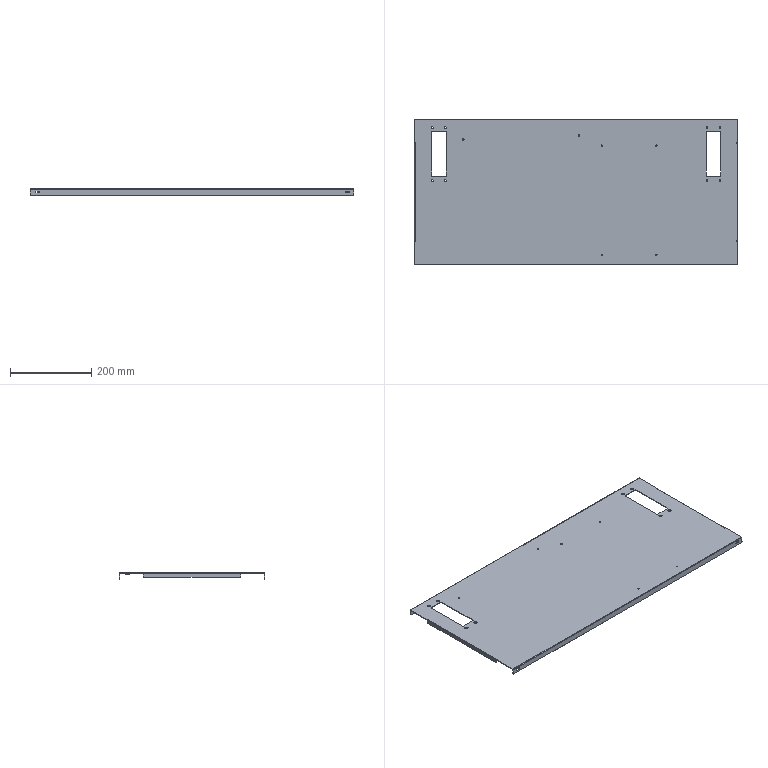Part | STEP file | Cabinet sheet-metal cover plate B | 1 solid | 147 faces | box 794.836 x 358 x 15 mm | volume 451787 mm3 | cylinder 76 | plane 71 | commonest cylinder face diameters 4 x16 4.2 x16 8.5 x16 3.3 x12 4.5 x8 0.02 x4